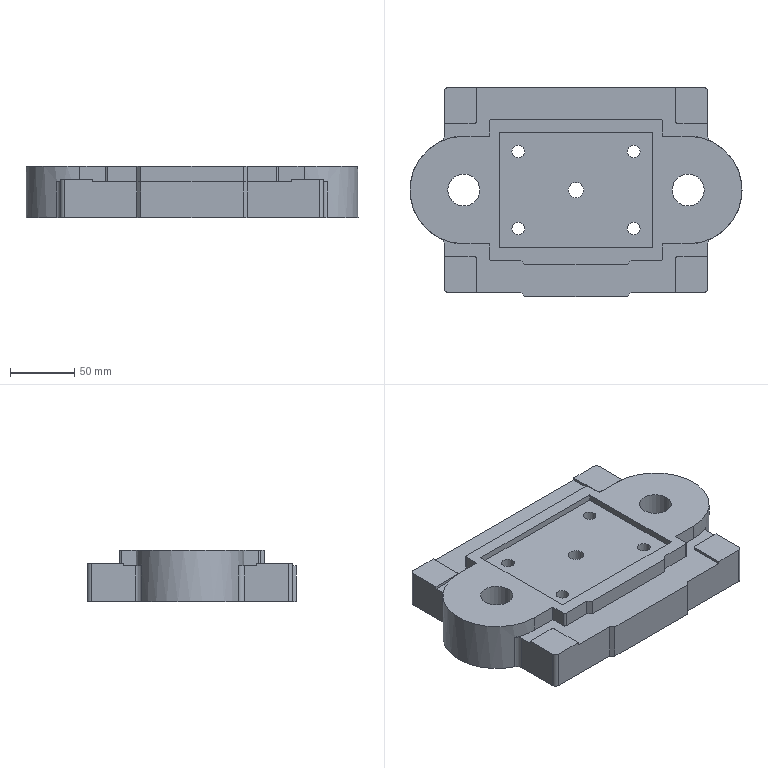Part | NX | features EXTRUDE 6, DATUM_CSYS 2, SKETCH 1 | 1 solid | 78 faces | box 259 x 163 x 40 mm | volume 1193308 mm3 | plane 49 | cylinder 29 | commonest cylinder face diameters 10 x8 3 x4 4 x4 6 x4 15 x4 25 x2